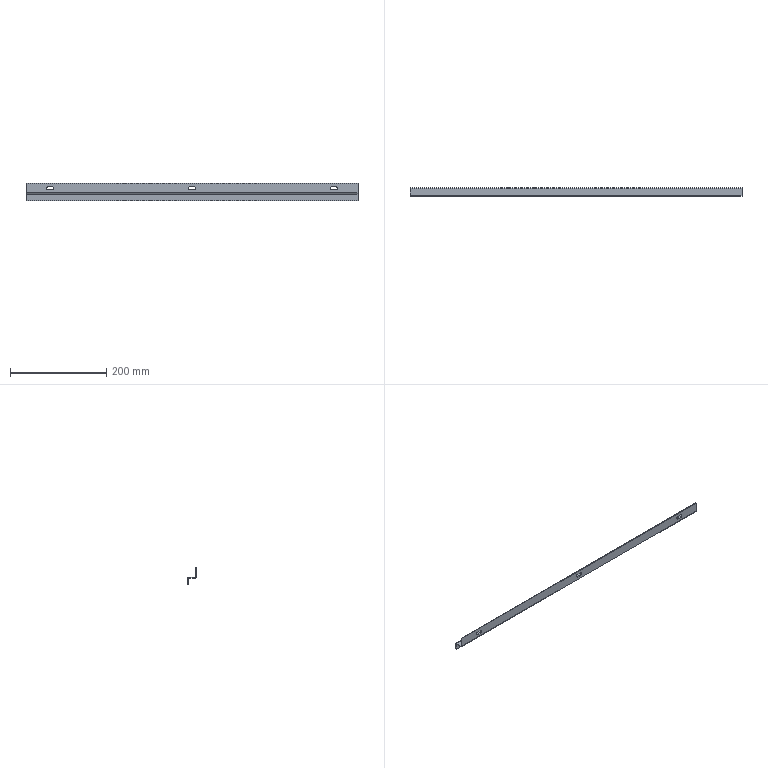Part | STEP file | 1 solid | 34 faces | box 690 x 18 x 35.5 mm | volume 51840 mm3 | plane 24 | cylinder 10 | commonest cylinder face diameters 7 x6 2 x2 5 x2